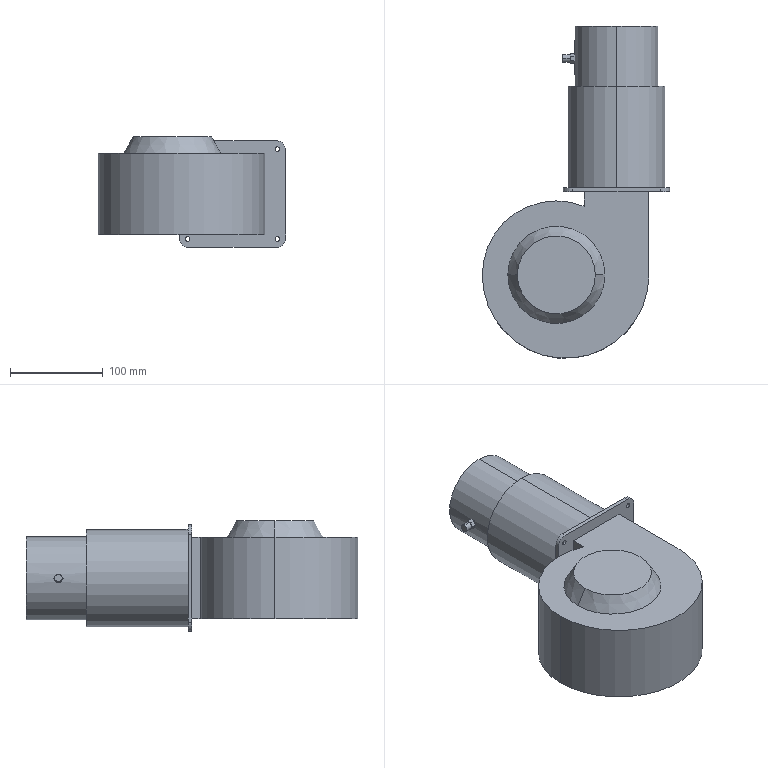Part | SolidWorks | features ICE 6, Extrusion 1 | 1 solid | 43 faces | box 202.5 x 359 x 119.5 mm | volume 3868562 mm3 | plane 21 | cylinder 20 | cone 2 | commonest cylinder face diameters 5 x8 20 x4 8 x2 90 x2 105 x2 160 x1
STEP:
#1=CARTESIAN_POINT('',(7.,234.,48.));
#2=VERTEX_POINT('',#1);
#3=CARTESIAN_POINT('',(7.,234.,40.));
#4=VERTEX_POINT('',#3);
#5=CARTESIAN_POINT('',(7.,234.,44.));
#6=DIRECTION('',(-1.,0.,0.));
#7=DIRECTION('',(0.,0.,1.));
#8=AXIS2_PLACEMENT_3D('',#5,#6,#7);
#9=CIRCLE('',#8,4.);
#10=EDGE_CURVE('',#2,#4,#9,.T.);
#11=ORIENTED_EDGE('',*,*,#10,.F.);
#12=CARTESIAN_POINT('',(15.,234.,48.));
#13=VERTEX_POINT('',#12);
#14=CARTESIAN_POINT('',(7.,234.,48.));
#15=DIRECTION('',(1.,0.,0.));
#16=VECTOR('',#15,1000.);
#17=LINE('',#14,#16);
#18=EDGE_CURVE('',#2,#13,#17,.T.);
#19=ORIENTED_EDGE('',*,*,#18,.T.);
#20=CARTESIAN_POINT('',(15.,234.,40.));
#21=VERTEX_POINT('',#20);
#22=CARTESIAN_POINT('',(15.,234.,44.));
#23=DIRECTION('',(-1.,0.,0.));
#24=DIRECTION('',(0.,0.,1.));
#25=AXIS2_PLACEMENT_3D('',#22,#23,#24);
#26=CIRCLE('',#25,4.);
#27=EDGE_CURVE('',#13,#21,#26,.T.);
#28=ORIENTED_EDGE('',*,*,#27,.T.);
#29=CARTESIAN_POINT('',(7.,234.,40.));
#30=DIRECTION('',(1.,0.,0.));
#31=VECTOR('',#30,1000.);
#32=LINE('',#29,#31);
#33=EDGE_CURVE('',#4,#21,#32,.T.);
#34=ORIENTED_EDGE('',*,*,#33,.F.);
#35=EDGE_LOOP('',(#11,#19,#28,#34));
#36=FACE_OUTER_BOUND('',#35,.T.);
#37=CARTESIAN_POINT('',(7.,234.,44.));
#38=DIRECTION('',(1.,0.,0.));
#39=DIRECTION('',(0.,0.,-1.));
#40=AXIS2_PLACEMENT_3D('',#37,#38,#39);
#41=CYLINDRICAL_SURFACE('',#40,4.);
#42=ADVANCED_FACE('',(#36),#41,.T.);
#43=CARTESIAN_POINT('',(65.,269.,89.));
#44=VERTEX_POINT('',#43);
#45=CARTESIAN_POINT('',(65.,269.,-1.));
#46=VERTEX_POINT('',#45);
#47=CARTESIAN_POINT('',(65.,269.,44.));
#48=DIRECTION('',(0.,1.,0.));
#49=DIRECTION('',(0.,0.,1.));
#50=AXIS2_PLACEMENT_3D('',#47,#48,#49);
#51=CIRCLE('',#50,45.);
#52=EDGE_CURVE('',#44,#46,#51,.T.);
#53=ORIENTED_EDGE('',*,*,#52,.F.);
#54=CARTESIAN_POINT('',(65.,204.,89.));
#55=VERTEX_POINT('',#54);
#56=CARTESIAN_POINT('',(65.,269.,89.));
#57=DIRECTION('',(0.,-1.,0.));
#58=VECTOR('',#57,1000.);
#59=LINE('',#56,#58);
#60=EDGE_CURVE('',#44,#55,#59,.T.);
#61=ORIENTED_EDGE('',*,*,#60,.T.);
#62=CARTESIAN_POINT('',(65.,204.,-1.));
#63=VERTEX_POINT('',#62);
#64=CARTESIAN_POINT('',(65.,204.,44.));
#65=DIRECTION('',(0.,1.,0.));
#66=DIRECTION('',(0.,0.,1.));
#67=AXIS2_PLACEMENT_3D('',#64,#65,#66);
#68=CIRCLE('',#67,45.);
#69=EDGE_CURVE('',#55,#63,#68,.T.);
#70=ORIENTED_EDGE('',*,*,#69,.T.);
#71=CARTESIAN_POINT('',(65.,269.,-1.));
#72=DIRECTION('',(0.,-1.,0.));
#73=VECTOR('',#72,1000.);
#74=LINE('',#71,#73);
#75=EDGE_CURVE('',#46,#63,#74,.T.);
#76=ORIENTED_EDGE('',*,*,#75,.F.);
#77=EDGE_LOOP('',(#53,#61,#70,#76));
#78=FACE_OUTER_BOUND('',#77,.T.);
#79=CARTESIAN_POINT('',(65.,269.,44.));
#80=DIRECTION('',(0.,-1.,0.));
#81=DIRECTION('',(0.,0.,-1.));
#82=AXIS2_PLACEMENT_3D('',#79,#80,#81);
#83=CYLINDRICAL_SURFACE('',#82,45.);
#84=ADVANCED_FACE('',(#78),#83,.T.);
#85=CARTESIAN_POINT('',(65.,204.,96.5));
#86=VERTEX_POINT('',#85);
#87=CARTESIAN_POINT('',(65.,204.,-8.5));
#88=VERTEX_POINT('',#87);
#89=CARTESIAN_POINT('',(65.,204.,44.));
#90=DIRECTION('',(0.,1.,0.));
#91=DIRECTION('',(0.,0.,1.));
#92=AXIS2_PLACEMENT_3D('',#89,#90,#91);
#93=CIRCLE('',#92,52.5);
#94=EDGE_CURVE('',#86,#88,#93,.T.);
#95=ORIENTED_EDGE('',*,*,#94,.F.);
#96=CARTESIAN_POINT('',(65.,94.,96.5));
#97=VERTEX_POINT('',#96);
#98=CARTESIAN_POINT('',(65.,204.,96.5));
#99=DIRECTION('',(0.,-1.,0.));
#100=VECTOR('',#99,1000.);
#101=LINE('',#98,#100);
#102=EDGE_CURVE('',#86,#97,#101,.T.);
#103=ORIENTED_EDGE('',*,*,#102,.T.);
#104=CARTESIAN_POINT('',(65.,94.,-8.5));
#105=VERTEX_POINT('',#104);
#106=CARTESIAN_POINT('',(65.,94.,44.));
#107=DIRECTION('',(0.,1.,0.));
#108=DIRECTION('',(0.,0.,-1.));
#109=AXIS2_PLACEMENT_3D('',#106,#107,#108);
#110=CIRCLE('',#109,52.5);
#111=EDGE_CURVE('',#97,#105,#110,.T.);
#112=ORIENTED_EDGE('',*,*,#111,.T.);
#113=CARTESIAN_POINT('',(65.,204.,-8.5));
#114=DIRECTION('',(0.,-1.,0.));
#115=VECTOR('',#114,1000.);
#116=LINE('',#113,#115);
#117=EDGE_CURVE('',#88,#105,#116,.T.);
#118=ORIENTED_EDGE('',*,*,#117,.F.);
#119=EDGE_LOOP('',(#95,#103,#112,#118));
#120=FACE_OUTER_BOUND('',#119,.T.);
#121=CARTESIAN_POINT('',(65.,204.,44.));
#122=DIRECTION('',(0.,-1.,0.));
#123=DIRECTION('',(0.,0.,-1.));
#124=AXIS2_PLACEMENT_3D('',#121,#122,#123);
#125=CYLINDRICAL_SURFACE('',#124,52.5);
#126=ADVANCED_FACE('',(#120),#125,.T.);
#127=CARTESIAN_POINT('',(113.5,94.,-7.));
#128=VERTEX_POINT('',#127);
#129=CARTESIAN_POINT('',(113.5,94.,-2.));
#130=VERTEX_POINT('',#129);
#131=CARTESIAN_POINT('',(113.5,94.,-4.5));
#132=DIRECTION('',(0.,1.,0.));
#133=DIRECTION('',(0.,0.,-1.));
#134=AXIS2_PLACEMENT_3D('',#131,#132,#133);
#135=CIRCLE('',#134,2.5);
#136=EDGE_CURVE('',#128,#130,#135,.T.);
#137=ORIENTED_EDGE('',*,*,#136,.T.);
#138=CARTESIAN_POINT('',(113.5,90.,-2.));
#139=VERTEX_POINT('',#138);
#140=CARTESIAN_POINT('',(113.5,94.,-2.));
#141=DIRECTION('',(0.,-1.,0.));
#142=VECTOR('',#141,1000.);
#143=LINE('',#140,#142);
#144=EDGE_CURVE('',#130,#139,#143,.T.);
#145=ORIENTED_EDGE('',*,*,#144,.T.);
#146=CARTESIAN_POINT('',(113.5,90.,-7.));
#147=VERTEX_POINT('',#146);
#148=CARTESIAN_POINT('',(113.5,90.,-4.5));
#149=DIRECTION('',(0.,1.,0.));
#150=DIRECTION('',(0.,0.,-1.));
#151=AXIS2_PLACEMENT_3D('',#148,#149,#150);
#152=CIRCLE('',#151,2.5);
#153=EDGE_CURVE('',#147,#139,#152,.T.);
#154=ORIENTED_EDGE('',*,*,#153,.F.);
#155=CARTESIAN_POINT('',(113.5,94.,-7.));
#156=DIRECTION('',(0.,-1.,0.));
#157=VECTOR('',#156,1000.);
#158=LINE('',#155,#157);
#159=EDGE_CURVE('',#128,#147,#158,.T.);
#160=ORIENTED_EDGE('',*,*,#159,.F.);
#161=EDGE_LOOP('',(#137,#145,#154,#160));
#162=FACE_OUTER_BOUND('',#161,.T.);
#163=CARTESIAN_POINT('',(113.5,94.,-4.5));
#164=DIRECTION('',(0.,-1.,0.));
#165=DIRECTION('',(0.,0.,-1.));
#166=AXIS2_PLACEMENT_3D('',#163,#164,#165);
#167=CYLINDRICAL_SURFACE('',#166,2.5);
#168=ADVANCED_FACE('',(#162),#167,.F.);
#169=CARTESIAN_POINT('',(113.5,94.,90.));
#170=VERTEX_POINT('',#169);
#171=CARTESIAN_POINT('',(113.5,94.,95.));
#172=VERTEX_POINT('',#171);
#173=CARTESIAN_POINT('',(113.5,94.,92.5));
#174=DIRECTION('',(0.,1.,0.));
#175=DIRECTION('',(0.,0.,1.));
#176=AXIS2_PLACEMENT_3D('',#173,#174,#175);
#177=CIRCLE('',#176,2.5);
#178=EDGE_CURVE('',#170,#172,#177,.T.);
#179=ORIENTED_EDGE('',*,*,#178,.T.);
#180=CARTESIAN_POINT('',(113.5,90.,95.));
#181=VERTEX_POINT('',#180);
#182=CARTESIAN_POINT('',(113.5,94.,95.));
#183=DIRECTION('',(0.,-1.,0.));
#184=VECTOR('',#183,1000.);
#185=LINE('',#182,#184);
#186=EDGE_CURVE('',#172,#181,#185,.T.);
#187=ORIENTED_EDGE('',*,*,#186,.T.);
#188=CARTESIAN_POINT('',(113.5,90.,90.));
#189=VERTEX_POINT('',#188);
#190=CARTESIAN_POINT('',(113.5,90.,92.5));
#191=DIRECTION('',(0.,1.,0.));
#192=DIRECTION('',(0.,0.,1.));
#193=AXIS2_PLACEMENT_3D('',#190,#191,#192);
#194=CIRCLE('',#193,2.5);
#195=EDGE_CURVE('',#189,#181,#194,.T.);
#196=ORIENTED_EDGE('',*,*,#195,.F.);
#197=CARTESIAN_POINT('',(113.5,94.,90.));
#198=DIRECTION('',(0.,-1.,0.));
#199=VECTOR('',#198,1000.);
#200=LINE('',#197,#199);
#201=EDGE_CURVE('',#170,#189,#200,.T.);
#202=ORIENTED_EDGE('',*,*,#201,.F.);
#203=EDGE_LOOP('',(#179,#187,#196,#202));
#204=FACE_OUTER_BOUND('',#203,.T.);
#205=CARTESIAN_POINT('',(113.5,94.,92.5));
#206=DIRECTION('',(0.,-1.,0.));
#207=DIRECTION('',(0.,0.,-1.));
#208=AXIS2_PLACEMENT_3D('',#205,#206,#207);
#209=CYLINDRICAL_SURFACE('',#208,2.5);
#210=ADVANCED_FACE('',(#204),#209,.F.);
#211=CARTESIAN_POINT('',(16.5,94.,90.));
#212=VERTEX_POINT('',#211);
#213=CARTESIAN_POINT('',(16.5,94.,95.));
#214=VERTEX_POINT('',#213);
#215=CARTESIAN_POINT('',(16.5,94.,92.5));
#216=DIRECTION('',(0.,1.,0.));
#217=DIRECTION('',(0.,0.,-1.));
#218=AXIS2_PLACEMENT_3D('',#215,#216,#217);
#219=CIRCLE('',#218,2.5);
#220=EDGE_CURVE('',#212,#214,#219,.T.);
#221=ORIENTED_EDGE('',*,*,#220,.T.);
#222=CARTESIAN_POINT('',(16.5,90.,95.));
#223=VERTEX_POINT('',#222);
#224=CARTESIAN_POINT('',(16.5,94.,95.));
#225=DIRECTION('',(0.,-1.,0.));
#226=VECTOR('',#225,1000.);
#227=LINE('',#224,#226);
#228=EDGE_CURVE('',#214,#223,#227,.T.);
#229=ORIENTED_EDGE('',*,*,#228,.T.);
#230=CARTESIAN_POINT('',(16.5,90.,90.));
#231=VERTEX_POINT('',#230);
#232=CARTESIAN_POINT('',(16.5,90.,92.5));
#233=DIRECTION('',(0.,1.,0.));
#234=DIRECTION('',(0.,0.,-1.));
#235=AXIS2_PLACEMENT_3D('',#232,#233,#234);
#236=CIRCLE('',#235,2.5);
#237=EDGE_CURVE('',#231,#223,#236,.T.);
#238=ORIENTED_EDGE('',*,*,#237,.F.);
#239=CARTESIAN_POINT('',(16.5,94.,90.));
#240=DIRECTION('',(0.,-1.,0.));
#241=VECTOR('',#240,1000.);
#242=LINE('',#239,#241);
#243=EDGE_CURVE('',#212,#231,#242,.T.);
#244=ORIENTED_EDGE('',*,*,#243,.F.);
#245=EDGE_LOOP('',(#221,#229,#238,#244));
#246=FACE_OUTER_BOUND('',#245,.T.);
#247=CARTESIAN_POINT('',(16.5,94.,92.5));
#248=DIRECTION('',(0.,-1.,0.));
#249=DIRECTION('',(0.,0.,-1.));
#250=AXIS2_PLACEMENT_3D('',#247,#248,#249);
#251=CYLINDRICAL_SURFACE('',#250,2.5);
#252=ADVANCED_FACE('',(#246),#251,.F.);
#253=CARTESIAN_POINT('',(16.5,94.,-7.));
#254=VERTEX_POINT('',#253);
#255=CARTESIAN_POINT('',(16.5,94.,-2.));
#256=VERTEX_POINT('',#255);
#257=CARTESIAN_POINT('',(16.5,94.,-4.5));
#258=DIRECTION('',(0.,1.,0.));
#259=DIRECTION('',(0.,0.,1.));
#260=AXIS2_PLACEMENT_3D('',#257,#258,#259);
#261=CIRCLE('',#260,2.5);
#262=EDGE_CURVE('',#254,#256,#261,.T.);
#263=ORIENTED_EDGE('',*,*,#262,.T.);
#264=CARTESIAN_POINT('',(16.5,90.,-2.));
#265=VERTEX_POINT('',#264);
#266=CARTESIAN_POINT('',(16.5,94.,-2.));
#267=DIRECTION('',(0.,-1.,0.));
#268=VECTOR('',#267,1000.);
#269=LINE('',#266,#268);
#270=EDGE_CURVE('',#256,#265,#269,.T.);
#271=ORIENTED_EDGE('',*,*,#270,.T.);
#272=CARTESIAN_POINT('',(16.5,90.,-7.));
#273=VERTEX_POINT('',#272);
#274=CARTESIAN_POINT('',(16.5,90.,-4.5));
#275=DIRECTION('',(0.,1.,0.));
#276=DIRECTION('',(0.,0.,1.));
#277=AXIS2_PLACEMENT_3D('',#274,#275,#276);
#278=CIRCLE('',#277,2.5);
#279=EDGE_CURVE('',#273,#265,#278,.T.);
#280=ORIENTED_EDGE('',*,*,#279,.F.);
#281=CARTESIAN_POINT('',(16.5,94.,-7.));
#282=DIRECTION('',(0.,-1.,0.));
#283=VECTOR('',#282,1000.);
#284=LINE('',#281,#283);
#285=EDGE_CURVE('',#254,#273,#284,.T.);
#286=ORIENTED_EDGE('',*,*,#285,.F.);
#287=EDGE_LOOP('',(#263,#271,#280,#286));
#288=FACE_OUTER_BOUND('',#287,.T.);
#289=CARTESIAN_POINT('',(16.5,94.,-4.5));
#290=DIRECTION('',(0.,-1.,0.));
#291=DIRECTION('',(0.,0.,-1.));
#292=AXIS2_PLACEMENT_3D('',#289,#290,#291);
#293=CYLINDRICAL_SURFACE('',#292,2.5);
#294=ADVANCED_FACE('',(#288),#293,.F.);
#295=CARTESIAN_POINT('',(-42.108,0.,106.));
#296=VERTEX_POINT('',#295);
#297=CARTESIAN_POINT('',(42.108,0.,106.));
#298=VERTEX_POINT('',#297);
#299=CARTESIAN_POINT('',(0.,0.,106.));
#300=DIRECTION('',(0.,0.,1.));
#301=DIRECTION('',(1.,0.,0.));
#302=AXIS2_PLACEMENT_3D('',#299,#300,#301);
#303=CIRCLE('',#302,42.108);
#304=EDGE_CURVE('',#296,#298,#303,.T.);
#305=ORIENTED_EDGE('',*,*,#304,.F.);
#306=CARTESIAN_POINT('',(-52.5,0.,88.));
#307=VERTEX_POINT('',#306);
#308=CARTESIAN_POINT('',(-52.5,0.,88.));
#309=DIRECTION('',(-0.5,0.,-0.866));
#310=VECTOR('',#309,1000.);
#311=LINE('',#308,#310);
#312=EDGE_CURVE('',#296,#307,#311,.T.);
#313=ORIENTED_EDGE('',*,*,#312,.T.);
#314=CARTESIAN_POINT('',(52.5,0.,88.));
#315=VERTEX_POINT('',#314);
#316=CARTESIAN_POINT('',(0.,0.,88.));
#317=DIRECTION('',(0.,0.,1.));
#318=DIRECTION('',(1.,0.,0.));
#319=AXIS2_PLACEMENT_3D('',#316,#317,#318);
#320=CIRCLE('',#319,52.5);
#321=EDGE_CURVE('',#307,#315,#320,.T.);
#322=ORIENTED_EDGE('',*,*,#321,.T.);
#323=CARTESIAN_POINT('',(52.5,0.,88.));
#324=DIRECTION('',(0.5,0.,-0.866));
#325=VECTOR('',#324,1000.);
#326=LINE('',#323,#325);
#327=EDGE_CURVE('',#298,#315,#326,.T.);
#328=ORIENTED_EDGE('',*,*,#327,.F.);
#329=EDGE_LOOP('',(#305,#313,#322,#328));
#330=FACE_OUTER_BOUND('',#329,.T.);
#331=CARTESIAN_POINT('',(0.,0.,88.));
#332=DIRECTION('',(0.,0.,-1.));
#333=DIRECTION('',(1.,0.,0.));
#334=AXIS2_PLACEMENT_3D('',#331,#332,#333);
#335=CONICAL_SURFACE('',#334,52.5,0.5236);
#336=ADVANCED_FACE('',(#330),#335,.T.);
#337=CARTESIAN_POINT('',(15.,236.5,48.33));
#338=VERTEX_POINT('',#337);
#339=CARTESIAN_POINT('',(15.,239.,44.));
#340=VERTEX_POINT('',#339);
#341=CARTESIAN_POINT('',(15.,236.5,48.33));
#342=DIRECTION('',(0.,0.5,-0.866));
#343=VECTOR('',#342,1000.);
#344=LINE('',#341,#343);
#345=EDGE_CURVE('',#338,#340,#344,.T.);
#346=ORIENTED_EDGE('',*,*,#345,.T.);
#347=CARTESIAN_POINT('',(15.,236.5,39.67));
#348=VERTEX_POINT('',#347);
#349=CARTESIAN_POINT('',(15.,239.,44.));
#350=DIRECTION('',(0.,-0.5,-0.866));
#351=VECTOR('',#350,1000.);
#352=LINE('',#349,#351);
#353=EDGE_CURVE('',#340,#348,#352,.T.);
#354=ORIENTED_EDGE('',*,*,#353,.T.);
#355=CARTESIAN_POINT('',(15.,231.5,39.67));
#356=VERTEX_POINT('',#355);
#357=CARTESIAN_POINT('',(15.,236.5,39.67));
#358=DIRECTION('',(0.,-1.,0.));
#359=VECTOR('',#358,1000.);
#360=LINE('',#357,#359);
#361=EDGE_CURVE('',#348,#356,#360,.T.);
#362=ORIENTED_EDGE('',*,*,#361,.T.);
#363=CARTESIAN_POINT('',(15.,229.,44.));
#364=VERTEX_POINT('',#363);
#365=CARTESIAN_POINT('',(15.,231.5,39.67));
#366=DIRECTION('',(0.,-0.5,0.866));
#367=VECTOR('',#366,1000.);
#368=LINE('',#365,#367);
#369=EDGE_CURVE('',#356,#364,#368,.T.);
#370=ORIENTED_EDGE('',*,*,#369,.T.);
#371=CARTESIAN_POINT('',(15.,231.5,48.33));
#372=VERTEX_POINT('',#371);
#373=CARTESIAN_POINT('',(15.,229.,44.));
#374=DIRECTION('',(0.,0.5,0.866));
#375=VECTOR('',#374,1000.);
#376=LINE('',#373,#375);
#377=EDGE_CURVE('',#364,#372,#376,.T.);
#378=ORIENTED_EDGE('',*,*,#377,.T.);
#379=CARTESIAN_POINT('',(15.,231.5,48.33));
#380=DIRECTION('',(0.,1.,0.));
#381=VECTOR('',#380,1000.);
#382=LINE('',#379,#381);
#383=EDGE_CURVE('',#372,#338,#382,.T.);
#384=ORIENTED_EDGE('',*,*,#383,.T.);
#385=EDGE_LOOP('',(#346,#354,#362,#370,#378,#384));
#386=FACE_OUTER_BOUND('',#385,.T.);
#387=CARTESIAN_POINT('',(15.,234.,44.));
#388=DIRECTION('',(-1.,0.,0.));
#389=DIRECTION('',(0.,0.,1.));
#390=AXIS2_PLACEMENT_3D('',#387,#388,#389);
#391=CIRCLE('',#390,4.);
#392=EDGE_CURVE('',#21,#13,#391,.T.);
#393=ORIENTED_EDGE('',*,*,#392,.F.);
#394=ORIENTED_EDGE('',*,*,#27,.F.);
#395=EDGE_LOOP('',(#393,#394));
#396=FACE_BOUND('',#395,.T.);
#397=CARTESIAN_POINT('',(15.,239.,44.));
#398=DIRECTION('',(-1.,0.,0.));
#399=DIRECTION('',(0.,0.,1.));
#400=AXIS2_PLACEMENT_3D('',#397,#398,#399);
#401=PLANE('',#400);
#402=ADVANCED_FACE('',(#386,#396),#401,.T.);
#403=CARTESIAN_POINT('',(65.,204.,44.));
#404=DIRECTION('',(0.,1.,0.));
#405=DIRECTION('',(0.,0.,1.));
#406=AXIS2_PLACEMENT_3D('',#403,#404,#405);
#407=CIRCLE('',#406,52.5);
#408=EDGE_CURVE('',#88,#86,#407,.T.);
#409=ORIENTED_EDGE('',*,*,#408,.T.);
#410=ORIENTED_EDGE('',*,*,#94,.T.);
#411=EDGE_LOOP('',(#409,#410));
#412=FACE_OUTER_BOUND('',#411,.T.);
#413=CARTESIAN_POINT('',(65.,204.,44.));
#414=DIRECTION('',(0.,1.,0.));
#415=DIRECTION('',(0.,0.,1.));
#416=AXIS2_PLACEMENT_3D('',#413,#414,#415);
#417=CIRCLE('',#416,45.);
#418=EDGE_CURVE('',#63,#55,#417,.T.);
#419=ORIENTED_EDGE('',*,*,#418,.F.);
#420=ORIENTED_EDGE('',*,*,#69,.F.);
#421=EDGE_LOOP('',(#419,#420));
#422=FACE_BOUND('',#421,.T.);
#423=CARTESIAN_POINT('',(65.,204.,44.));
#424=DIRECTION('',(0.,1.,0.));
#425=DIRECTION('',(0.,0.,1.));
#426=AXIS2_PLACEMENT_3D('',#423,#424,#425);
#427=PLANE('',#426);
#428=ADVANCED_FACE('',(#412,#422),#427,.T.);
#429=ORIENTED_EDGE('',*,*,#136,.F.);
#430=CARTESIAN_POINT('',(113.5,94.,-4.5));
#431=DIRECTION('',(0.,1.,0.));
#432=DIRECTION('',(0.,0.,-1.));
#433=AXIS2_PLACEMENT_3D('',#430,#431,#432);
#434=CIRCLE('',#433,2.5);
#435=EDGE_CURVE('',#130,#128,#434,.T.);
#436=ORIENTED_EDGE('',*,*,#435,.F.);
#437=EDGE_LOOP('',(#429,#436));
#438=FACE_BOUND('',#437,.T.);
#439=ORIENTED_EDGE('',*,*,#220,.F.);
#440=CARTESIAN_POINT('',(16.5,94.,92.5));
#441=DIRECTION('',(0.,1.,0.));
#442=DIRECTION('',(0.,0.,-1.));
#443=AXIS2_PLACEMENT_3D('',#440,#441,#442);
#444=CIRCLE('',#443,2.5);
#445=EDGE_CURVE('',#214,#212,#444,.T.);
#446=ORIENTED_EDGE('',*,*,#445,.F.);
#447=EDGE_LOOP('',(#439,#446));
#448=FACE_BOUND('',#447,.T.);
#449=CARTESIAN_POINT('',(122.5,94.,-3.5));
#450=VERTEX_POINT('',#449);
#451=CARTESIAN_POINT('',(112.5,94.,-13.5));
#452=VERTEX_POINT('',#451);
#453=CARTESIAN_POINT('',(112.5,94.,-3.5));
#454=DIRECTION('',(0.,1.,0.));
#455=DIRECTION('',(0.,0.,-1.));
#456=AXIS2_PLACEMENT_3D('',#453,#454,#455);
#457=CIRCLE('',#456,10.);
#458=EDGE_CURVE('',#450,#452,#457,.T.);
#459=ORIENTED_EDGE('',*,*,#458,.T.);
#460=CARTESIAN_POINT('',(17.5,94.,-13.5));
#461=VERTEX_POINT('',#460);
#462=CARTESIAN_POINT('',(17.5,94.,-13.5));
#463=DIRECTION('',(-1.,0.,0.));
#464=VECTOR('',#463,1000.);
#465=LINE('',#462,#464);
#466=EDGE_CURVE('',#452,#461,#465,.T.);
#467=ORIENTED_EDGE('',*,*,#466,.T.);
#468=CARTESIAN_POINT('',(7.5,94.,-3.5));
#469=VERTEX_POINT('',#468);
#470=CARTESIAN_POINT('',(17.5,94.,-3.5));
#471=DIRECTION('',(0.,1.,0.));
#472=DIRECTION('',(0.,0.,-1.));
#473=AXIS2_PLACEMENT_3D('',#470,#471,#472);
#474=CIRCLE('',#473,10.);
#475=EDGE_CURVE('',#461,#469,#474,.T.);
#476=ORIENTED_EDGE('',*,*,#475,.T.);
#477=CARTESIAN_POINT('',(7.5,94.,91.5));
#478=VERTEX_POINT('',#477);
#479=CARTESIAN_POINT('',(7.5,94.,-3.5));
#480=DIRECTION('',(0.,0.,1.));
#481=VECTOR('',#480,1000.);
#482=LINE('',#479,#481);
#483=EDGE_CURVE('',#469,#478,#482,.T.);
#484=ORIENTED_EDGE('',*,*,#483,.T.);
#485=CARTESIAN_POINT('',(17.5,94.,101.5));
#486=VERTEX_POINT('',#485);
#487=CARTESIAN_POINT('',(17.5,94.,91.5));
#488=DIRECTION('',(0.,1.,0.));
#489=DIRECTION('',(0.,0.,-1.));
#490=AXIS2_PLACEMENT_3D('',#487,#488,#489);
#491=CIRCLE('',#490,10.);
#492=EDGE_CURVE('',#478,#486,#491,.T.);
#493=ORIENTED_EDGE('',*,*,#492,.T.);
#494=CARTESIAN_POINT('',(112.5,94.,101.5));
#495=VERTEX_POINT('',#494);
#496=CARTESIAN_POINT('',(17.5,94.,101.5));
#497=DIRECTION('',(1.,0.,0.));
#498=VECTOR('',#497,1000.);
#499=LINE('',#496,#498);
#500=EDGE_CURVE('',#486,#495,#499,.T.);
#501=ORIENTED_EDGE('',*,*,#500,.T.);
#502=CARTESIAN_POINT('',(122.5,94.,91.5));
#503=VERTEX_POINT('',#502);
#504=CARTESIAN_POINT('',(112.5,94.,91.5));
#505=DIRECTION('',(0.,1.,0.));
#506=DIRECTION('',(0.,0.,-1.));
#507=AXIS2_PLACEMENT_3D('',#504,#505,#506);
#508=CIRCLE('',#507,10.);
#509=EDGE_CURVE('',#495,#503,#508,.T.);
#510=ORIENTED_EDGE('',*,*,#509,.T.);
#511=CARTESIAN_POINT('',(122.5,94.,-3.5));
#512=DIRECTION('',(0.,0.,-1.));
#513=VECTOR('',#512,1000.);
#514=LINE('',#511,#513);
#515=EDGE_CURVE('',#503,#450,#514,.T.);
#516=ORIENTED_EDGE('',*,*,#515,.T.);
#517=EDGE_LOOP('',(#459,#467,#476,#484,#493,#501,#510,#516));
#518=FACE_OUTER_BOUND('',#517,.T.);
#519=ORIENTED_EDGE('',*,*,#262,.F.);
#520=CARTESIAN_POINT('',(16.5,94.,-4.5));
#521=DIRECTION('',(0.,1.,0.));
#522=DIRECTION('',(0.,0.,1.));
#523=AXIS2_PLACEMENT_3D('',#520,#521,#522);
#524=CIRCLE('',#523,2.5);
#525=EDGE_CURVE('',#256,#254,#524,.T.);
#526=ORIENTED_EDGE('',*,*,#525,.F.);
#527=EDGE_LOOP('',(#519,#526));
#528=FACE_BOUND('',#527,.T.);
#529=ORIENTED_EDGE('',*,*,#178,.F.);
#530=CARTESIAN_POINT('',(113.5,94.,92.5));
#531=DIRECTION('',(0.,1.,0.));
#532=DIRECTION('',(0.,0.,1.));
#533=AXIS2_PLACEMENT_3D('',#530,#531,#532);
#534=CIRCLE('',#533,2.5);
#535=EDGE_CURVE('',#172,#170,#534,.T.);
#536=ORIENTED_EDGE('',*,*,#535,.F.);
#537=EDGE_LOOP('',(#529,#536));
#538=FACE_BOUND('',#537,.T.);
#539=CARTESIAN_POINT('',(65.,94.,44.));
#540=DIRECTION('',(0.,1.,0.));
#541=DIRECTION('',(0.,0.,-1.));
#542=AXIS2_PLACEMENT_3D('',#539,#540,#541);
#543=CIRCLE('',#542,52.5);
#544=EDGE_CURVE('',#105,#97,#543,.T.);
#545=ORIENTED_EDGE('',*,*,#544,.F.);
#546=ORIENTED_EDGE('',*,*,#111,.F.);
#547=EDGE_LOOP('',(#545,#546));
#548=FACE_BOUND('',#547,.T.);
#549=CARTESIAN_POINT('',(112.5,94.,-3.5));
#550=DIRECTION('',(0.,-1.,0.));
#551=DIRECTION('',(0.,0.,-1.));
#552=AXIS2_PLACEMENT_3D('',#549,#550,#551);
#553=PLANE('',#552);
#554=ADVANCED_FACE('',(#438,#448,#518,#528,#538,#548),#553,.F.);
#555=CARTESIAN_POINT('',(100.,90.,88.));
#556=VERTEX_POINT('',#555);
#557=CARTESIAN_POINT('',(30.,90.,88.));
#558=VERTEX_POINT('',#557);
#559=CARTESIAN_POINT('',(30.,90.,88.));
#560=DIRECTION('',(-1.,0.,0.));
#561=VECTOR('',#560,1000.);
#562=LINE('',#559,#561);
#563=EDGE_CURVE('',#556,#558,#562,.T.);
#564=ORIENTED_EDGE('',*,*,#563,.T.);
#565=CARTESIAN_POINT('',(30.,74.162,88.));
#566=VERTEX_POINT('',#565);
#567=CARTESIAN_POINT('',(30.,90.,88.));
#568=DIRECTION('',(0.,-1.,0.));
#569=VECTOR('',#568,1000.);
#570=LINE('',#567,#569);
#571=EDGE_CURVE('',#558,#566,#570,.T.);
#572=ORIENTED_EDGE('',*,*,#571,.T.);
#573=CARTESIAN_POINT('',(-80.,0.,88.));
#574=VERTEX_POINT('',#573);
#575=CARTESIAN_POINT('',(0.,0.,88.));
#576=DIRECTION('',(0.,0.,1.));
#577=DIRECTION('',(1.,0.,0.));
#578=AXIS2_PLACEMENT_3D('',#575,#576,#577);
#579=CIRCLE('',#578,80.);
#580=EDGE_CURVE('',#566,#574,#579,.T.);
#581=ORIENTED_EDGE('',*,*,#580,.T.);
#582=CARTESIAN_POINT('',(100.,0.,88.));
#583=VERTEX_POINT('',#582);
#584=CARTESIAN_POINT('',(10.,0.,88.));
#585=DIRECTION('',(0.,0.,1.));
#586=DIRECTION('',(1.,0.,0.));
#587=AXIS2_PLACEMENT_3D('',#584,#585,#586);
#588=CIRCLE('',#587,90.);
#589=EDGE_CURVE('',#574,#583,#588,.T.);
#590=ORIENTED_EDGE('',*,*,#589,.T.);
#591=CARTESIAN_POINT('',(100.,0.,88.));
#592=DIRECTION('',(0.,1.,0.));
#593=VECTOR('',#592,1000.);
#594=LINE('',#591,#593);
#595=EDGE_CURVE('',#583,#556,#594,.T.);
#596=ORIENTED_EDGE('',*,*,#595,.T.);
#597=EDGE_LOOP('',(#564,#572,#581,#590,#596));
#598=FACE_OUTER_BOUND('',#597,.T.);
#599=CARTESIAN_POINT('',(0.,0.,88.));
#600=DIRECTION('',(0.,0.,1.));
#601=DIRECTION('',(1.,0.,0.));
#602=AXIS2_PLACEMENT_3D('',#599,#600,#601);
#603=CIRCLE('',#602,52.5);
#604=EDGE_CURVE('',#315,#307,#603,.T.);
#605=ORIENTED_EDGE('',*,*,#604,.F.);
#606=ORIENTED_EDGE('',*,*,#321,.F.);
#607=EDGE_LOOP('',(#605,#606));
#608=FACE_BOUND('',#607,.T.);
#609=CARTESIAN_POINT('',(10.,0.,88.));
#610=DIRECTION('',(0.,0.,1.));
#611=DIRECTION('',(1.,0.,0.));
#612=AXIS2_PLACEMENT_3D('',#609,#610,#611);
#613=PLANE('',#612);
#614=ADVANCED_FACE('',(#598,#608),#613,.T.);
#615=CARTESIAN_POINT('',(30.,90.,0.));
#616=VERTEX_POINT('',#615);
#617=CARTESIAN_POINT('',(30.,74.162,0.));
#618=VERTEX_POINT('',#617);
#619=CARTESIAN_POINT('',(30.,90.,0.));
#620=DIRECTION('',(0.,-1.,0.));
#621=VECTOR('',#620,1000.);
#622=LINE('',#619,#621);
#623=EDGE_CURVE('',#616,#618,#622,.T.);
#624=ORIENTED_EDGE('',*,*,#623,.T.);
#625=CARTESIAN_POINT('',(30.,74.162,88.));
#626=DIRECTION('',(0.,0.,-1.));
#627=VECTOR('',#626,1000.);
#628=LINE('',#625,#627);
#629=EDGE_CURVE('',#566,#618,#628,.T.);
#630=ORIENTED_EDGE('',*,*,#629,.F.);
#631=ORIENTED_EDGE('',*,*,#571,.F.);
#632=CARTESIAN_POINT('',(30.,90.,88.));
#633=DIRECTION('',(0.,0.,-1.));
#634=VECTOR('',#633,1000.);
#635=LINE('',#632,#634);
#636=EDGE_CURVE('',#558,#616,#635,.T.);
#637=ORIENTED_EDGE('',*,*,#636,.T.);
#638=EDGE_LOOP('',(#624,#630,#631,#637));
#639=FACE_OUTER_BOUND('',#638,.T.);
#640=CARTESIAN_POINT('',(30.,90.,88.));
#641=DIRECTION('',(1.,0.,0.));
#642=DIRECTION('',(0.,0.,-1.));
#643=AXIS2_PLACEMENT_3D('',#640,#641,#642);
#644=PLANE('',#643);
#645=ADVANCED_FACE('',(#639),#644,.F.);
#646=CARTESIAN_POINT('',(-80.,0.,0.));
#647=VERTEX_POINT('',#646);
#648=CARTESIAN_POINT('',(0.,0.,0.));
#649=DIRECTION('',(0.,0.,1.));
#650=DIRECTION('',(1.,0.,0.));
#651=AXIS2_PLACEMENT_3D('',#648,#649,#650);
#652=CIRCLE('',#651,80.);
#653=EDGE_CURVE('',#618,#647,#652,.T.);
#654=ORIENTED_EDGE('',*,*,#653,.T.);
#655=CARTESIAN_POINT('',(-80.,0.,88.));
#656=DIRECTION('',(0.,0.,-1.));
#657=VECTOR('',#656,1000.);
#658=LINE('',#655,#657);
#659=EDGE_CURVE('',#574,#647,#658,.T.);
#660=ORIENTED_EDGE('',*,*,#659,.F.);
#661=ORIENTED_EDGE('',*,*,#580,.F.);
#662=ORIENTED_EDGE('',*,*,#629,.T.);
#663=EDGE_LOOP('',(#654,#660,#661,#662));
#664=FACE_OUTER_BOUND('',#663,.T.);
#665=CARTESIAN_POINT('',(0.,0.,88.));
#666=DIRECTION('',(0.,0.,-1.));
#667=DIRECTION('',(-1.,0.,0.));
#668=AXIS2_PLACEMENT_3D('',#665,#666,#667);
#669=CYLINDRICAL_SURFACE('',#668,80.);
#670=ADVANCED_FACE('',(#664),#669,.T.);
#671=CARTESIAN_POINT('',(100.,0.,0.));
#672=VERTEX_POINT('',#671);
#673=CARTESIAN_POINT('',(10.,0.,0.));
#674=DIRECTION('',(0.,0.,1.));
#675=DIRECTION('',(1.,0.,0.));
#676=AXIS2_PLACEMENT_3D('',#673,#674,#675);
#677=CIRCLE('',#676,90.);
#678=EDGE_CURVE('',#647,#672,#677,.T.);
#679=ORIENTED_EDGE('',*,*,#678,.T.);
#680=CARTESIAN_POINT('',(100.,0.,88.));
#681=DIRECTION('',(0.,0.,-1.));
#682=VECTOR('',#681,1000.);
#683=LINE('',#680,#682);
#684=EDGE_CURVE('',#583,#672,#683,.T.);
#685=ORIENTED_EDGE('',*,*,#684,.F.);
#686=ORIENTED_EDGE('',*,*,#589,.F.);
#687=ORIENTED_EDGE('',*,*,#659,.T.);
#688=EDGE_LOOP('',(#679,#685,#686,#687));
#689=FACE_OUTER_BOUND('',#688,.T.);
#690=CARTESIAN_POINT('',(10.,0.,88.));
#691=DIRECTION('',(0.,0.,-1.));
#692=DIRECTION('',(-1.,0.,0.));
#693=AXIS2_PLACEMENT_3D('',#690,#691,#692);
#694=CYLINDRICAL_SURFACE('',#693,90.);
#695=ADVANCED_FACE('',(#689),#694,.T.);
#696=CARTESIAN_POINT('',(100.,90.,0.));
#697=VERTEX_POINT('',#696);
#698=CARTESIAN_POINT('',(100.,0.,0.));
#699=DIRECTION('',(0.,1.,0.));
#700=VECTOR('',#699,1000.);
#701=LINE('',#698,#700);
#702=EDGE_CURVE('',#672,#697,#701,.T.);
#703=ORIENTED_EDGE('',*,*,#702,.T.);
#704=CARTESIAN_POINT('',(100.,90.,88.));
#705=DIRECTION('',(0.,0.,-1.));
#706=VECTOR('',#705,1000.);
#707=LINE('',#704,#706);
#708=EDGE_CURVE('',#556,#697,#707,.T.);
#709=ORIENTED_EDGE('',*,*,#708,.F.);
#710=ORIENTED_EDGE('',*,*,#595,.F.);
#711=ORIENTED_EDGE('',*,*,#684,.T.);
#712=EDGE_LOOP('',(#703,#709,#710,#711));
#713=FACE_OUTER_BOUND('',#712,.T.);
#714=CARTESIAN_POINT('',(100.,0.,88.));
#715=DIRECTION('',(-1.,0.,0.));
#716=DIRECTION('',(0.,0.,1.));
#717=AXIS2_PLACEMENT_3D('',#714,#715,#716);
#718=PLANE('',#717);
#719=ADVANCED_FACE('',(#713),#718,.F.);
#720=CARTESIAN_POINT('',(30.,90.,0.));
#721=DIRECTION('',(-1.,0.,0.));
#722=VECTOR('',#721,1000.);
#723=LINE('',#720,#722);
#724=EDGE_CURVE('',#697,#616,#723,.T.);
#725=ORIENTED_EDGE('',*,*,#724,.F.);
#726=ORIENTED_EDGE('',*,*,#702,.F.);
#727=ORIENTED_EDGE('',*,*,#678,.F.);
#728=ORIENTED_EDGE('',*,*,#653,.F.);
#729=ORIENTED_EDGE('',*,*,#623,.F.);
#730=EDGE_LOOP('',(#725,#726,#727,#728,#729));
#731=FACE_OUTER_BOUND('',#730,.T.);
#732=CARTESIAN_POINT('',(10.,0.,0.));
#733=DIRECTION('',(0.,0.,1.));
#734=DIRECTION('',(1.,0.,0.));
#735=AXIS2_PLACEMENT_3D('',#732,#733,#734);
#736=PLANE('',#735);
#737=ADVANCED_FACE('',(#731),#736,.F.);
#738=ORIENTED_EDGE('',*,*,#312,.F.);
#739=CARTESIAN_POINT('',(0.,0.,106.));
#740=DIRECTION('',(0.,0.,1.));
#741=DIRECTION('',(1.,0.,0.));
#742=AXIS2_PLACEMENT_3D('',#739,#740,#741);
#743=CIRCLE('',#742,42.108);
#744=EDGE_CURVE('',#298,#296,#743,.T.);
#745=ORIENTED_EDGE('',*,*,#744,.F.);
#746=ORIENTED_EDGE('',*,*,#327,.T.);
#747=ORIENTED_EDGE('',*,*,#604,.T.);
#748=EDGE_LOOP('',(#738,#745,#746,#747));
#749=FACE_OUTER_BOUND('',#748,.T.);
#750=CARTESIAN_POINT('',(0.,0.,88.));
#751=DIRECTION('',(0.,0.,-1.));
#752=DIRECTION('',(1.,0.,0.));
#753=AXIS2_PLACEMENT_3D('',#750,#751,#752);
#754=CONICAL_SURFACE('',#753,52.5,0.5236);
#755=ADVANCED_FACE('',(#749),#754,.T.);
#756=ORIENTED_EDGE('',*,*,#744,.T.);
#757=ORIENTED_EDGE('',*,*,#304,.T.);
#758=EDGE_LOOP('',(#756,#757));
#759=FACE_OUTER_BOUND('',#758,.T.);
#760=CARTESIAN_POINT('',(0.,0.,106.));
#761=DIRECTION('',(0.,0.,1.));
#762=DIRECTION('',(1.,0.,0.));
#763=AXIS2_PLACEMENT_3D('',#760,#761,#762);
#764=PLANE('',#763);
#765=ADVANCED_FACE('',(#759),#764,.T.);
#766=ORIENTED_EDGE('',*,*,#636,.F.);
#767=ORIENTED_EDGE('',*,*,#563,.F.);
#768=ORIENTED_EDGE('',*,*,#708,.T.);
#769=ORIENTED_EDGE('',*,*,#724,.T.);
#770=EDGE_LOOP('',(#766,#767,#768,#769));
#771=FACE_BOUND('',#770,.T.);
#772=ORIENTED_EDGE('',*,*,#195,.T.);
#773=CARTESIAN_POINT('',(113.5,90.,92.5));
#774=DIRECTION('',(0.,1.,0.));
#775=DIRECTION('',(0.,0.,1.));
#776=AXIS2_PLACEMENT_3D('',#773,#774,#775);
#777=CIRCLE('',#776,2.5);
#778=EDGE_CURVE('',#181,#189,#777,.T.);
#779=ORIENTED_EDGE('',*,*,#778,.T.);
#780=EDGE_LOOP('',(#772,#779));
#781=FACE_BOUND('',#780,.T.);
#782=ORIENTED_EDGE('',*,*,#279,.T.);
#783=CARTESIAN_POINT('',(16.5,90.,-4.5));
#784=DIRECTION('',(0.,1.,0.));
#785=DIRECTION('',(0.,0.,1.));
#786=AXIS2_PLACEMENT_3D('',#783,#784,#785);
#787=CIRCLE('',#786,2.5);
#788=EDGE_CURVE('',#265,#273,#787,.T.);
#789=ORIENTED_EDGE('',*,*,#788,.T.);
#790=EDGE_LOOP('',(#782,#789));
#791=FACE_BOUND('',#790,.T.);
#792=CARTESIAN_POINT('',(122.5,90.,-3.5));
#793=VERTEX_POINT('',#792);
#794=CARTESIAN_POINT('',(112.5,90.,-13.5));
#795=VERTEX_POINT('',#794);
#796=CARTESIAN_POINT('',(112.5,90.,-3.5));
#797=DIRECTION('',(0.,1.,0.));
#798=DIRECTION('',(0.,0.,-1.));
#799=AXIS2_PLACEMENT_3D('',#796,#797,#798);
#800=CIRCLE('',#799,10.);
#801=EDGE_CURVE('',#793,#795,#800,.T.);
#802=ORIENTED_EDGE('',*,*,#801,.F.);
#803=CARTESIAN_POINT('',(122.5,90.,91.5));
#804=VERTEX_POINT('',#803);
#805=CARTESIAN_POINT('',(122.5,90.,-3.5));
#806=DIRECTION('',(0.,0.,-1.));
#807=VECTOR('',#806,1000.);
#808=LINE('',#805,#807);
#809=EDGE_CURVE('',#804,#793,#808,.T.);
#810=ORIENTED_EDGE('',*,*,#809,.F.);
#811=CARTESIAN_POINT('',(112.5,90.,101.5));
#812=VERTEX_POINT('',#811);
#813=CARTESIAN_POINT('',(112.5,90.,91.5));
#814=DIRECTION('',(0.,1.,0.));
#815=DIRECTION('',(0.,0.,-1.));
#816=AXIS2_PLACEMENT_3D('',#813,#814,#815);
#817=CIRCLE('',#816,10.);
#818=EDGE_CURVE('',#812,#804,#817,.T.);
#819=ORIENTED_EDGE('',*,*,#818,.F.);
#820=CARTESIAN_POINT('',(17.5,90.,101.5));
#821=VERTEX_POINT('',#820);
#822=CARTESIAN_POINT('',(17.5,90.,101.5));
#823=DIRECTION('',(1.,0.,0.));
#824=VECTOR('',#823,1000.);
#825=LINE('',#822,#824);
#826=EDGE_CURVE('',#821,#812,#825,.T.);
#827=ORIENTED_EDGE('',*,*,#826,.F.);
#828=CARTESIAN_POINT('',(7.5,90.,91.5));
#829=VERTEX_POINT('',#828);
#830=CARTESIAN_POINT('',(17.5,90.,91.5));
#831=DIRECTION('',(0.,1.,0.));
#832=DIRECTION('',(0.,0.,-1.));
#833=AXIS2_PLACEMENT_3D('',#830,#831,#832);
#834=CIRCLE('',#833,10.);
#835=EDGE_CURVE('',#829,#821,#834,.T.);
#836=ORIENTED_EDGE('',*,*,#835,.F.);
#837=CARTESIAN_POINT('',(7.5,90.,-3.5));
#838=VERTEX_POINT('',#837);
#839=CARTESIAN_POINT('',(7.5,90.,-3.5));
#840=DIRECTION('',(0.,0.,1.));
#841=VECTOR('',#840,1000.);
#842=LINE('',#839,#841);
#843=EDGE_CURVE('',#838,#829,#842,.T.);
#844=ORIENTED_EDGE('',*,*,#843,.F.);
#845=CARTESIAN_POINT('',(17.5,90.,-13.5));
#846=VERTEX_POINT('',#845);
#847=CARTESIAN_POINT('',(17.5,90.,-3.5));
#848=DIRECTION('',(0.,1.,0.));
#849=DIRECTION('',(0.,0.,-1.));
#850=AXIS2_PLACEMENT_3D('',#847,#848,#849);
#851=CIRCLE('',#850,10.);
#852=EDGE_CURVE('',#846,#838,#851,.T.);
#853=ORIENTED_EDGE('',*,*,#852,.F.);
#854=CARTESIAN_POINT('',(17.5,90.,-13.5));
#855=DIRECTION('',(-1.,0.,0.));
#856=VECTOR('',#855,1000.);
#857=LINE('',#854,#856);
#858=EDGE_CURVE('',#795,#846,#857,.T.);
#859=ORIENTED_EDGE('',*,*,#858,.F.);
#860=EDGE_LOOP('',(#802,#810,#819,#827,#836,#844,#853,#859));
#861=FACE_OUTER_BOUND('',#860,.T.);
#862=ORIENTED_EDGE('',*,*,#237,.T.);
#863=CARTESIAN_POINT('',(16.5,90.,92.5));
#864=DIRECTION('',(0.,1.,0.));
#865=DIRECTION('',(0.,0.,-1.));
#866=AXIS2_PLACEMENT_3D('',#863,#864,#865);
#867=CIRCLE('',#866,2.5);
#868=EDGE_CURVE('',#223,#231,#867,.T.);
#869=ORIENTED_EDGE('',*,*,#868,.T.);
#870=EDGE_LOOP('',(#862,#869));
#871=FACE_BOUND('',#870,.T.);
#872=ORIENTED_EDGE('',*,*,#153,.T.);
#873=CARTESIAN_POINT('',(113.5,90.,-4.5));
#874=DIRECTION('',(0.,1.,0.));
#875=DIRECTION('',(0.,0.,-1.));
#876=AXIS2_PLACEMENT_3D('',#873,#874,#875);
#877=CIRCLE('',#876,2.5);
#878=EDGE_CURVE('',#139,#147,#877,.T.);
#879=ORIENTED_EDGE('',*,*,#878,.T.);
#880=EDGE_LOOP('',(#872,#879));
#881=FACE_BOUND('',#880,.T.);
#882=CARTESIAN_POINT('',(112.5,90.,-3.5));
#883=DIRECTION('',(0.,-1.,0.));
#884=DIRECTION('',(0.,0.,-1.));
#885=AXIS2_PLACEMENT_3D('',#882,#883,#884);
#886=PLANE('',#885);
#887=ADVANCED_FACE('',(#771,#781,#791,#861,#871,#881),#886,.T.);
#888=ORIENTED_EDGE('',*,*,#801,.T.);
#889=CARTESIAN_POINT('',(112.5,94.,-13.5));
#890=DIRECTION('',(0.,-1.,0.));
#891=VECTOR('',#890,1000.);
#892=LINE('',#889,#891);
#893=EDGE_CURVE('',#452,#795,#892,.T.);
#894=ORIENTED_EDGE('',*,*,#893,.F.);
#895=ORIENTED_EDGE('',*,*,#458,.F.);
#896=CARTESIAN_POINT('',(122.5,94.,-3.5));
#897=DIRECTION('',(0.,-1.,0.));
#898=VECTOR('',#897,1000.);
#899=LINE('',#896,#898);
#900=EDGE_CURVE('',#450,#793,#899,.T.);
#901=ORIENTED_EDGE('',*,*,#900,.T.);
#902=EDGE_LOOP('',(#888,#894,#895,#901));
#903=FACE_OUTER_BOUND('',#902,.T.);
#904=CARTESIAN_POINT('',(112.5,94.,-3.5));
#905=DIRECTION('',(0.,-1.,0.));
#906=DIRECTION('',(0.,0.,-1.));
#907=AXIS2_PLACEMENT_3D('',#904,#905,#906);
#908=CYLINDRICAL_SURFACE('',#907,10.);
#909=ADVANCED_FACE('',(#903),#908,.T.);
#910=ORIENTED_EDGE('',*,*,#858,.T.);
#911=CARTESIAN_POINT('',(17.5,94.,-13.5));
#912=DIRECTION('',(0.,-1.,0.));
#913=VECTOR('',#912,1000.);
#914=LINE('',#911,#913);
#915=EDGE_CURVE('',#461,#846,#914,.T.);
#916=ORIENTED_EDGE('',*,*,#915,.F.);
#917=ORIENTED_EDGE('',*,*,#466,.F.);
#918=ORIENTED_EDGE('',*,*,#893,.T.);
#919=EDGE_LOOP('',(#910,#916,#917,#918));
#920=FACE_OUTER_BOUND('',#919,.T.);
#921=CARTESIAN_POINT('',(17.5,94.,-13.5));
#922=DIRECTION('',(0.,0.,1.));
#923=DIRECTION('',(1.,0.,0.));
#924=AXIS2_PLACEMENT_3D('',#921,#922,#923);
#925=PLANE('',#924);
#926=ADVANCED_FACE('',(#920),#925,.F.);
#927=ORIENTED_EDGE('',*,*,#852,.T.);
#928=CARTESIAN_POINT('',(7.5,94.,-3.5));
#929=DIRECTION('',(0.,-1.,0.));
#930=VECTOR('',#929,1000.);
#931=LINE('',#928,#930);
#932=EDGE_CURVE('',#469,#838,#931,.T.);
#933=ORIENTED_EDGE('',*,*,#932,.F.);
#934=ORIENTED_EDGE('',*,*,#475,.F.);
#935=ORIENTED_EDGE('',*,*,#915,.T.);
#936=EDGE_LOOP('',(#927,#933,#934,#935));
#937=FACE_OUTER_BOUND('',#936,.T.);
#938=CARTESIAN_POINT('',(17.5,94.,-3.5));
#939=DIRECTION('',(0.,-1.,0.));
#940=DIRECTION('',(0.,0.,-1.));
#941=AXIS2_PLACEMENT_3D('',#938,#939,#940);
#942=CYLINDRICAL_SURFACE('',#941,10.);
#943=ADVANCED_FACE('',(#937),#942,.T.);
#944=ORIENTED_EDGE('',*,*,#843,.T.);
#945=CARTESIAN_POINT('',(7.5,94.,91.5));
#946=DIRECTION('',(0.,-1.,0.));
#947=VECTOR('',#946,1000.);
#948=LINE('',#945,#947);
#949=EDGE_CURVE('',#478,#829,#948,.T.);
#950=ORIENTED_EDGE('',*,*,#949,.F.);
#951=ORIENTED_EDGE('',*,*,#483,.F.);
#952=ORIENTED_EDGE('',*,*,#932,.T.);
#953=EDGE_LOOP('',(#944,#950,#951,#952));
#954=FACE_OUTER_BOUND('',#953,.T.);
#955=CARTESIAN_POINT('',(7.5,94.,-3.5));
#956=DIRECTION('',(1.,0.,0.));
#957=DIRECTION('',(0.,0.,-1.));
#958=AXIS2_PLACEMENT_3D('',#955,#956,#957);
#959=PLANE('',#958);
#960=ADVANCED_FACE('',(#954),#959,.F.);
#961=ORIENTED_EDGE('',*,*,#835,.T.);
#962=CARTESIAN_POINT('',(17.5,94.,101.5));
#963=DIRECTION('',(0.,-1.,0.));
#964=VECTOR('',#963,1000.);
#965=LINE('',#962,#964);
#966=EDGE_CURVE('',#486,#821,#965,.T.);
#967=ORIENTED_EDGE('',*,*,#966,.F.);
#968=ORIENTED_EDGE('',*,*,#492,.F.);
#969=ORIENTED_EDGE('',*,*,#949,.T.);
#970=EDGE_LOOP('',(#961,#967,#968,#969));
#971=FACE_OUTER_BOUND('',#970,.T.);
#972=CARTESIAN_POINT('',(17.5,94.,91.5));
#973=DIRECTION('',(0.,-1.,0.));
#974=DIRECTION('',(0.,0.,-1.));
#975=AXIS2_PLACEMENT_3D('',#972,#973,#974);
#976=CYLINDRICAL_SURFACE('',#975,10.);
#977=ADVANCED_FACE('',(#971),#976,.T.);
#978=ORIENTED_EDGE('',*,*,#826,.T.);
#979=CARTESIAN_POINT('',(112.5,94.,101.5));
#980=DIRECTION('',(0.,-1.,0.));
#981=VECTOR('',#980,1000.);
#982=LINE('',#979,#981);
#983=EDGE_CURVE('',#495,#812,#982,.T.);
#984=ORIENTED_EDGE('',*,*,#983,.F.);
#985=ORIENTED_EDGE('',*,*,#500,.F.);
#986=ORIENTED_EDGE('',*,*,#966,.T.);
#987=EDGE_LOOP('',(#978,#984,#985,#986));
#988=FACE_OUTER_BOUND('',#987,.T.);
#989=CARTESIAN_POINT('',(17.5,94.,101.5));
#990=DIRECTION('',(0.,0.,-1.));
#991=DIRECTION('',(-1.,0.,0.));
#992=AXIS2_PLACEMENT_3D('',#989,#990,#991);
#993=PLANE('',#992);
#994=ADVANCED_FACE('',(#988),#993,.F.);
#995=ORIENTED_EDGE('',*,*,#818,.T.);
#996=CARTESIAN_POINT('',(122.5,94.,91.5));
#997=DIRECTION('',(0.,-1.,0.));
#998=VECTOR('',#997,1000.);
#999=LINE('',#996,#998);
#1000=EDGE_CURVE('',#503,#804,#999,.T.);
#1001=ORIENTED_EDGE('',*,*,#1000,.F.);
#1002=ORIENTED_EDGE('',*,*,#509,.F.);
#1003=ORIENTED_EDGE('',*,*,#983,.T.);
#1004=EDGE_LOOP('',(#995,#1001,#1002,#1003));
#1005=FACE_OUTER_BOUND('',#1004,.T.);
#1006=CARTESIAN_POINT('',(112.5,94.,91.5));
#1007=DIRECTION('',(0.,-1.,0.));
#1008=DIRECTION('',(0.,0.,-1.));
#1009=AXIS2_PLACEMENT_3D('',#1006,#1007,#1008);
#1010=CYLINDRICAL_SURFACE('',#1009,10.);
#1011=ADVANCED_FACE('',(#1005),#1010,.T.);
#1012=ORIENTED_EDGE('',*,*,#809,.T.);
#1013=ORIENTED_EDGE('',*,*,#900,.F.);
#1014=ORIENTED_EDGE('',*,*,#515,.F.);
#1015=ORIENTED_EDGE('',*,*,#1000,.T.);
#1016=EDGE_LOOP('',(#1012,#1013,#1014,#1015));
#1017=FACE_OUTER_BOUND('',#1016,.T.);
#1018=CARTESIAN_POINT('',(122.5,94.,-3.5));
#1019=DIRECTION('',(-1.,0.,0.));
#1020=DIRECTION('',(0.,0.,1.));
#1021=AXIS2_PLACEMENT_3D('',#1018,#1019,#1020);
#1022=PLANE('',#1021);
#1023=ADVANCED_FACE('',(#1017),#1022,.F.);
#1024=ORIENTED_EDGE('',*,*,#270,.F.);
#1025=ORIENTED_EDGE('',*,*,#525,.T.);
#1026=ORIENTED_EDGE('',*,*,#285,.T.);
#1027=ORIENTED_EDGE('',*,*,#788,.F.);
#1028=EDGE_LOOP('',(#1024,#1025,#1026,#1027));
#1029=FACE_OUTER_BOUND('',#1028,.T.);
#1030=CARTESIAN_POINT('',(16.5,94.,-4.5));
#1031=DIRECTION('',(0.,-1.,0.));
#1032=DIRECTION('',(0.,0.,-1.));
#1033=AXIS2_PLACEMENT_3D('',#1030,#1031,#1032);
#1034=CYLINDRICAL_SURFACE('',#1033,2.5);
#1035=ADVANCED_FACE('',(#1029),#1034,.F.);
#1036=ORIENTED_EDGE('',*,*,#228,.F.);
#1037=ORIENTED_EDGE('',*,*,#445,.T.);
#1038=ORIENTED_EDGE('',*,*,#243,.T.);
#1039=ORIENTED_EDGE('',*,*,#868,.F.);
#1040=EDGE_LOOP('',(#1036,#1037,#1038,#1039));
#1041=FACE_OUTER_BOUND('',#1040,.T.);
#1042=CARTESIAN_POINT('',(16.5,94.,92.5));
#1043=DIRECTION('',(0.,-1.,0.));
#1044=DIRECTION('',(0.,0.,-1.));
#1045=AXIS2_PLACEMENT_3D('',#1042,#1043,#1044);
#1046=CYLINDRICAL_SURFACE('',#1045,2.5);
#1047=ADVANCED_FACE('',(#1041),#1046,.F.);
#1048=ORIENTED_EDGE('',*,*,#186,.F.);
#1049=ORIENTED_EDGE('',*,*,#535,.T.);
#1050=ORIENTED_EDGE('',*,*,#201,.T.);
#1051=ORIENTED_EDGE('',*,*,#778,.F.);
#1052=EDGE_LOOP('',(#1048,#1049,#1050,#1051));
#1053=FACE_OUTER_BOUND('',#1052,.T.);
#1054=CARTESIAN_POINT('',(113.5,94.,92.5));
#1055=DIRECTION('',(0.,-1.,0.));
#1056=DIRECTION('',(0.,0.,-1.));
#1057=AXIS2_PLACEMENT_3D('',#1054,#1055,#1056);
#1058=CYLINDRICAL_SURFACE('',#1057,2.5);
#1059=ADVANCED_FACE('',(#1053),#1058,.F.);
#1060=ORIENTED_EDGE('',*,*,#144,.F.);
#1061=ORIENTED_EDGE('',*,*,#435,.T.);
#1062=ORIENTED_EDGE('',*,*,#159,.T.);
#1063=ORIENTED_EDGE('',*,*,#878,.F.);
#1064=EDGE_LOOP('',(#1060,#1061,#1062,#1063));
#1065=FACE_OUTER_BOUND('',#1064,.T.);
#1066=CARTESIAN_POINT('',(113.5,94.,-4.5));
#1067=DIRECTION('',(0.,-1.,0.));
#1068=DIRECTION('',(0.,0.,-1.));
#1069=AXIS2_PLACEMENT_3D('',#1066,#1067,#1068);
#1070=CYLINDRICAL_SURFACE('',#1069,2.5);
#1071=ADVANCED_FACE('',(#1065),#1070,.F.);
#1072=ORIENTED_EDGE('',*,*,#102,.F.);
#1073=ORIENTED_EDGE('',*,*,#408,.F.);
#1074=ORIENTED_EDGE('',*,*,#117,.T.);
#1075=ORIENTED_EDGE('',*,*,#544,.T.);
#1076=EDGE_LOOP('',(#1072,#1073,#1074,#1075));
#1077=FACE_OUTER_BOUND('',#1076,.T.);
#1078=CARTESIAN_POINT('',(65.,204.,44.));
#1079=DIRECTION('',(0.,-1.,0.));
#1080=DIRECTION('',(0.,0.,-1.));
#1081=AXIS2_PLACEMENT_3D('',#1078,#1079,#1080);
#1082=CYLINDRICAL_SURFACE('',#1081,52.5);
#1083=ADVANCED_FACE('',(#1077),#1082,.T.);
#1084=ORIENTED_EDGE('',*,*,#60,.F.);
#1085=CARTESIAN_POINT('',(65.,269.,44.));
#1086=DIRECTION('',(0.,1.,0.));
#1087=DIRECTION('',(0.,0.,1.));
#1088=AXIS2_PLACEMENT_3D('',#1085,#1086,#1087);
#1089=CIRCLE('',#1088,45.);
#1090=EDGE_CURVE('',#46,#44,#1089,.T.);
#1091=ORIENTED_EDGE('',*,*,#1090,.F.);
#1092=ORIENTED_EDGE('',*,*,#75,.T.);
#1093=ORIENTED_EDGE('',*,*,#418,.T.);
#1094=EDGE_LOOP('',(#1084,#1091,#1092,#1093));
#1095=FACE_OUTER_BOUND('',#1094,.T.);
#1096=CARTESIAN_POINT('',(20.209,236.5,39.67));
#1097=VERTEX_POINT('',#1096);
#1098=CARTESIAN_POINT('',(20.,239.,44.));
#1099=VERTEX_POINT('',#1098);
#1100=CARTESIAN_POINT('',(20.209,236.5,39.67));
#1101=CARTESIAN_POINT('',(20.07,237.331,41.109));
#1102=CARTESIAN_POINT('',(20.,238.165,42.554));
#1103=CARTESIAN_POINT('',(20.,239.,44.));
#1104=(BOUNDED_CURVE()B_SPLINE_CURVE(3,(#1100,#1101,#1102,#1103),.UNSPECIFIED.,.F.,.F.)B_SPLINE_CURVE_WITH_KNOTS((4,4),(1.474,1.571),.UNSPECIFIED.)CURVE()GEOMETRIC_REPRESENTATION_ITEM()RATIONAL_B_SPLINE_CURVE((1.,0.9992,0.9992,1.))REPRESENTATION_ITEM(''));
#1105=EDGE_CURVE('',#1097,#1099,#1104,.T.);
#1106=ORIENTED_EDGE('',*,*,#1105,.T.);
#1107=CARTESIAN_POINT('',(20.209,236.5,48.33));
#1108=VERTEX_POINT('',#1107);
#1109=CARTESIAN_POINT('',(20.,239.,44.));
#1110=CARTESIAN_POINT('',(20.,238.165,45.446));
#1111=CARTESIAN_POINT('',(20.07,237.331,46.891));
#1112=CARTESIAN_POINT('',(20.209,236.5,48.33));
#1113=(BOUNDED_CURVE()B_SPLINE_CURVE(3,(#1109,#1110,#1111,#1112),.UNSPECIFIED.,.F.,.F.)B_SPLINE_CURVE_WITH_KNOTS((4,4),(4.712,4.809),.UNSPECIFIED.)CURVE()GEOMETRIC_REPRESENTATION_ITEM()RATIONAL_B_SPLINE_CURVE((1.,0.9992,0.9992,1.))REPRESENTATION_ITEM(''));
#1114=EDGE_CURVE('',#1099,#1108,#1113,.T.);
#1115=ORIENTED_EDGE('',*,*,#1114,.T.);
#1116=CARTESIAN_POINT('',(20.209,231.5,48.33));
#1117=VERTEX_POINT('',#1116);
#1118=CARTESIAN_POINT('',(20.209,269.,48.33));
#1119=DIRECTION('',(0.,-1.,0.));
#1120=VECTOR('',#1119,1000.);
#1121=LINE('',#1118,#1120);
#1122=EDGE_CURVE('',#1108,#1117,#1121,.T.);
#1123=ORIENTED_EDGE('',*,*,#1122,.T.);
#1124=CARTESIAN_POINT('',(20.,229.,44.));
#1125=VERTEX_POINT('',#1124);
#1126=CARTESIAN_POINT('',(20.209,231.5,48.33));
#1127=CARTESIAN_POINT('',(20.07,230.669,46.891));
#1128=CARTESIAN_POINT('',(20.,229.835,45.446));
#1129=CARTESIAN_POINT('',(20.,229.,44.));
#1130=(BOUNDED_CURVE()B_SPLINE_CURVE(3,(#1126,#1127,#1128,#1129),.UNSPECIFIED.,.F.,.F.)B_SPLINE_CURVE_WITH_KNOTS((4,4),(4.616,4.712),.UNSPECIFIED.)CURVE()GEOMETRIC_REPRESENTATION_ITEM()RATIONAL_B_SPLINE_CURVE((1.,0.9992,0.9992,1.))REPRESENTATION_ITEM(''));
#1131=EDGE_CURVE('',#1117,#1125,#1130,.T.);
#1132=ORIENTED_EDGE('',*,*,#1131,.T.);
#1133=CARTESIAN_POINT('',(20.209,231.5,39.67));
#1134=VERTEX_POINT('',#1133);
#1135=CARTESIAN_POINT('',(20.,229.,44.));
#1136=CARTESIAN_POINT('',(20.,229.835,42.554));
#1137=CARTESIAN_POINT('',(20.07,230.669,41.109));
#1138=CARTESIAN_POINT('',(20.209,231.5,39.67));
#1139=(BOUNDED_CURVE()B_SPLINE_CURVE(3,(#1135,#1136,#1137,#1138),.UNSPECIFIED.,.F.,.F.)B_SPLINE_CURVE_WITH_KNOTS((4,4),(1.571,1.667),.UNSPECIFIED.)CURVE()GEOMETRIC_REPRESENTATION_ITEM()RATIONAL_B_SPLINE_CURVE((1.,0.9992,0.9992,1.))REPRESENTATION_ITEM(''));
#1140=EDGE_CURVE('',#1125,#1134,#1139,.T.);
#1141=ORIENTED_EDGE('',*,*,#1140,.T.);
#1142=CARTESIAN_POINT('',(20.209,269.,39.67));
#1143=DIRECTION('',(0.,1.,0.));
#1144=VECTOR('',#1143,1000.);
#1145=LINE('',#1142,#1144);
#1146=EDGE_CURVE('',#1134,#1097,#1145,.T.);
#1147=ORIENTED_EDGE('',*,*,#1146,.T.);
#1148=EDGE_LOOP('',(#1106,#1115,#1123,#1132,#1141,#1147));
#1149=FACE_BOUND('',#1148,.T.);
#1150=CARTESIAN_POINT('',(65.,269.,44.));
#1151=DIRECTION('',(0.,-1.,0.));
#1152=DIRECTION('',(0.,0.,-1.));
#1153=AXIS2_PLACEMENT_3D('',#1150,#1151,#1152);
#1154=CYLINDRICAL_SURFACE('',#1153,45.);
#1155=ADVANCED_FACE('',(#1095,#1149),#1154,.T.);
#1156=ORIENTED_EDGE('',*,*,#1090,.T.);
#1157=ORIENTED_EDGE('',*,*,#52,.T.);
#1158=EDGE_LOOP('',(#1156,#1157));
#1159=FACE_OUTER_BOUND('',#1158,.T.);
#1160=CARTESIAN_POINT('',(65.,269.,44.));
#1161=DIRECTION('',(0.,1.,0.));
#1162=DIRECTION('',(0.,0.,1.));
#1163=AXIS2_PLACEMENT_3D('',#1160,#1161,#1162);
#1164=PLANE('',#1163);
#1165=ADVANCED_FACE('',(#1159),#1164,.T.);
#1166=ORIENTED_EDGE('',*,*,#1114,.F.);
#1167=CARTESIAN_POINT('',(25.,239.,44.));
#1168=DIRECTION('',(-1.,0.,0.));
#1169=VECTOR('',#1168,1000.);
#1170=LINE('',#1167,#1169);
#1171=EDGE_CURVE('',#1099,#340,#1170,.T.);
#1172=ORIENTED_EDGE('',*,*,#1171,.T.);
#1173=ORIENTED_EDGE('',*,*,#345,.F.);
#1174=CARTESIAN_POINT('',(25.,236.5,48.33));
#1175=DIRECTION('',(-1.,0.,0.));
#1176=VECTOR('',#1175,1000.);
#1177=LINE('',#1174,#1176);
#1178=EDGE_CURVE('',#1108,#338,#1177,.T.);
#1179=ORIENTED_EDGE('',*,*,#1178,.F.);
#1180=EDGE_LOOP('',(#1166,#1172,#1173,#1179));
#1181=FACE_OUTER_BOUND('',#1180,.T.);
#1182=CARTESIAN_POINT('',(25.,236.5,48.33));
#1183=DIRECTION('',(0.,0.866,0.5));
#1184=DIRECTION('',(0.,-0.5,0.866));
#1185=AXIS2_PLACEMENT_3D('',#1182,#1183,#1184);
#1186=PLANE('',#1185);
#1187=ADVANCED_FACE('',(#1181),#1186,.T.);
#1188=ORIENTED_EDGE('',*,*,#1122,.F.);
#1189=ORIENTED_EDGE('',*,*,#1178,.T.);
#1190=ORIENTED_EDGE('',*,*,#383,.F.);
#1191=CARTESIAN_POINT('',(25.,231.5,48.33));
#1192=DIRECTION('',(-1.,0.,0.));
#1193=VECTOR('',#1192,1000.);
#1194=LINE('',#1191,#1193);
#1195=EDGE_CURVE('',#1117,#372,#1194,.T.);
#1196=ORIENTED_EDGE('',*,*,#1195,.F.);
#1197=EDGE_LOOP('',(#1188,#1189,#1190,#1196));
#1198=FACE_OUTER_BOUND('',#1197,.T.);
#1199=CARTESIAN_POINT('',(25.,231.5,48.33));
#1200=DIRECTION('',(0.,0.,1.));
#1201=DIRECTION('',(1.,0.,0.));
#1202=AXIS2_PLACEMENT_3D('',#1199,#1200,#1201);
#1203=PLANE('',#1202);
#1204=ADVANCED_FACE('',(#1198),#1203,.T.);
#1205=ORIENTED_EDGE('',*,*,#1131,.F.);
#1206=ORIENTED_EDGE('',*,*,#1195,.T.);
#1207=ORIENTED_EDGE('',*,*,#377,.F.);
#1208=CARTESIAN_POINT('',(25.,229.,44.));
#1209=DIRECTION('',(-1.,0.,0.));
#1210=VECTOR('',#1209,1000.);
#1211=LINE('',#1208,#1210);
#1212=EDGE_CURVE('',#1125,#364,#1211,.T.);
#1213=ORIENTED_EDGE('',*,*,#1212,.F.);
#1214=EDGE_LOOP('',(#1205,#1206,#1207,#1213));
#1215=FACE_OUTER_BOUND('',#1214,.T.);
#1216=CARTESIAN_POINT('',(25.,229.,44.));
#1217=DIRECTION('',(0.,-0.866,0.5));
#1218=DIRECTION('',(0.,-0.5,-0.866));
#1219=AXIS2_PLACEMENT_3D('',#1216,#1217,#1218);
#1220=PLANE('',#1219);
#1221=ADVANCED_FACE('',(#1215),#1220,.T.);
#1222=ORIENTED_EDGE('',*,*,#1140,.F.);
#1223=ORIENTED_EDGE('',*,*,#1212,.T.);
#1224=ORIENTED_EDGE('',*,*,#369,.F.);
#1225=CARTESIAN_POINT('',(25.,231.5,39.67));
#1226=DIRECTION('',(-1.,0.,0.));
#1227=VECTOR('',#1226,1000.);
#1228=LINE('',#1225,#1227);
#1229=EDGE_CURVE('',#1134,#356,#1228,.T.);
#1230=ORIENTED_EDGE('',*,*,#1229,.F.);
#1231=EDGE_LOOP('',(#1222,#1223,#1224,#1230));
#1232=FACE_OUTER_BOUND('',#1231,.T.);
#1233=CARTESIAN_POINT('',(25.,231.5,39.67));
#1234=DIRECTION('',(0.,-0.866,-0.5));
#1235=DIRECTION('',(0.,0.5,-0.866));
#1236=AXIS2_PLACEMENT_3D('',#1233,#1234,#1235);
#1237=PLANE('',#1236);
#1238=ADVANCED_FACE('',(#1232),#1237,.T.);
#1239=ORIENTED_EDGE('',*,*,#1146,.F.);
#1240=ORIENTED_EDGE('',*,*,#1229,.T.);
#1241=ORIENTED_EDGE('',*,*,#361,.F.);
#1242=CARTESIAN_POINT('',(25.,236.5,39.67));
#1243=DIRECTION('',(-1.,0.,0.));
#1244=VECTOR('',#1243,1000.);
#1245=LINE('',#1242,#1244);
#1246=EDGE_CURVE('',#1097,#348,#1245,.T.);
#1247=ORIENTED_EDGE('',*,*,#1246,.F.);
#1248=EDGE_LOOP('',(#1239,#1240,#1241,#1247));
#1249=FACE_OUTER_BOUND('',#1248,.T.);
#1250=CARTESIAN_POINT('',(25.,236.5,39.67));
#1251=DIRECTION('',(0.,0.,-1.));
#1252=DIRECTION('',(-1.,0.,0.));
#1253=AXIS2_PLACEMENT_3D('',#1250,#1251,#1252);
#1254=PLANE('',#1253);
#1255=ADVANCED_FACE('',(#1249),#1254,.T.);
#1256=ORIENTED_EDGE('',*,*,#1105,.F.);
#1257=ORIENTED_EDGE('',*,*,#1246,.T.);
#1258=ORIENTED_EDGE('',*,*,#353,.F.);
#1259=ORIENTED_EDGE('',*,*,#1171,.F.);
#1260=EDGE_LOOP('',(#1256,#1257,#1258,#1259));
#1261=FACE_OUTER_BOUND('',#1260,.T.);
#1262=CARTESIAN_POINT('',(25.,239.,44.));
#1263=DIRECTION('',(0.,0.866,-0.5));
#1264=DIRECTION('',(0.,0.5,0.866));
#1265=AXIS2_PLACEMENT_3D('',#1262,#1263,#1264);
#1266=PLANE('',#1265);
#1267=ADVANCED_FACE('',(#1261),#1266,.T.);
#1268=ORIENTED_EDGE('',*,*,#18,.F.);
#1269=CARTESIAN_POINT('',(7.,234.,44.));
#1270=DIRECTION('',(-1.,0.,0.));
#1271=DIRECTION('',(0.,0.,1.));
#1272=AXIS2_PLACEMENT_3D('',#1269,#1270,#1271);
#1273=CIRCLE('',#1272,4.);
#1274=EDGE_CURVE('',#4,#2,#1273,.T.);
#1275=ORIENTED_EDGE('',*,*,#1274,.F.);
#1276=ORIENTED_EDGE('',*,*,#33,.T.);
#1277=ORIENTED_EDGE('',*,*,#392,.T.);
#1278=EDGE_LOOP('',(#1268,#1275,#1276,#1277));
#1279=FACE_OUTER_BOUND('',#1278,.T.);
#1280=CARTESIAN_POINT('',(7.,234.,44.));
#1281=DIRECTION('',(1.,0.,0.));
#1282=DIRECTION('',(0.,0.,-1.));
#1283=AXIS2_PLACEMENT_3D('',#1280,#1281,#1282);
#1284=CYLINDRICAL_SURFACE('',#1283,4.);
#1285=ADVANCED_FACE('',(#1279),#1284,.T.);
#1286=ORIENTED_EDGE('',*,*,#1274,.T.);
#1287=ORIENTED_EDGE('',*,*,#10,.T.);
#1288=EDGE_LOOP('',(#1286,#1287));
#1289=FACE_OUTER_BOUND('',#1288,.T.);
#1290=CARTESIAN_POINT('',(7.,234.,44.));
#1291=DIRECTION('',(-1.,0.,0.));
#1292=DIRECTION('',(0.,0.,1.));
#1293=AXIS2_PLACEMENT_3D('',#1290,#1291,#1292);
#1294=PLANE('',#1293);
#1295=ADVANCED_FACE('',(#1289),#1294,.T.);
#1296=CLOSED_SHELL('',(#42,#84,#126,#168,#210,#252,#294,#336,#402,#428,#554,#614,#645,#670,#695,#719,#737,#755,#765,#887,#909,#926,#943,#960,#977,#994,#1011,#1023,#1035,#1047,#1059,#1071,#1083,#1155,#1165,#1187,#1204,#1221,#1238,#1255,#1267,#1285,#1295));
#1297=MANIFOLD_SOLID_BREP('',#1296);
#1298=CARTESIAN_POINT('',(0.,0.,0.));
#1299=DIRECTION('',(0.,0.,1.));
#1300=DIRECTION('',(1.,0.,0.));
#1301=AXIS2_PLACEMENT_3D('',#1298,#1299,#1300);
#1302=(LENGTH_UNIT()NAMED_UNIT(*)SI_UNIT(.MILLI.,.METRE.));
#1303=UNCERTAINTY_MEASURE_WITH_UNIT(LENGTH_MEASURE(0.00001),#1302,'','');
#1304=(NAMED_UNIT(*)PLANE_ANGLE_UNIT()SI_UNIT($,.RADIAN.));
#1305=(NAMED_UNIT(*)SI_UNIT($,.STERADIAN.)SOLID_ANGLE_UNIT());
#1306=(GEOMETRIC_REPRESENTATION_CONTEXT(3)GLOBAL_UNCERTAINTY_ASSIGNED_CONTEXT((#1303))GLOBAL_UNIT_ASSIGNED_CONTEXT((#1302,#1304,#1305))REPRESENTATION_CONTEXT('',''));
#1307=ADVANCED_BREP_SHAPE_REPRESENTATION('',(#1297,#1301),#1306);